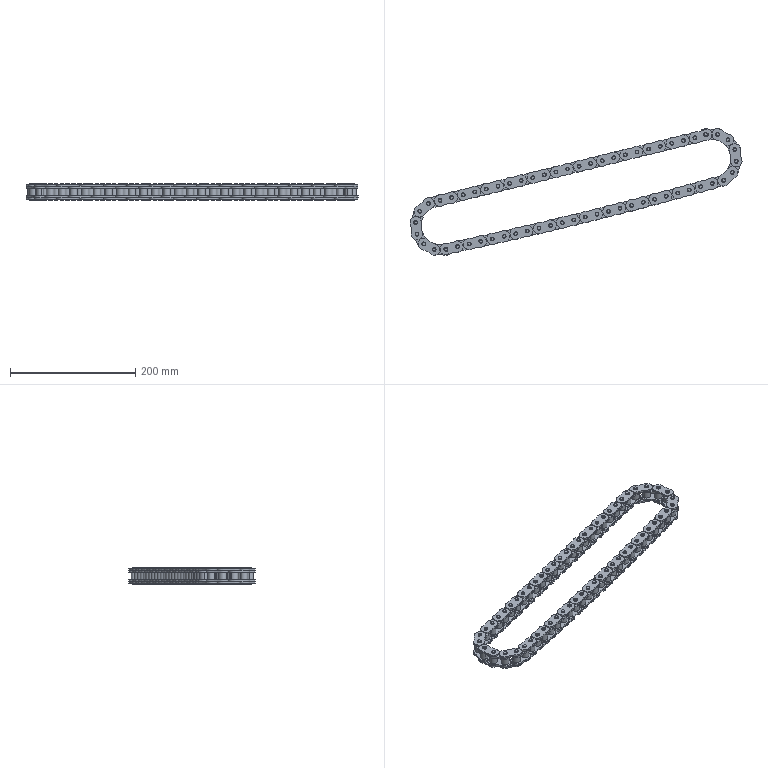Part | SolidWorks | features BaseBody 90 | 90 solids | 1800 faces | box 530.16 x 202.19 x 26.9 mm | volume 270718 mm3 | cylinder 1200 | plane 360 | cone 240 | commonest cylinder face diameters 5.96 x480 18.08 x360 83.184 x240 11.91 x120